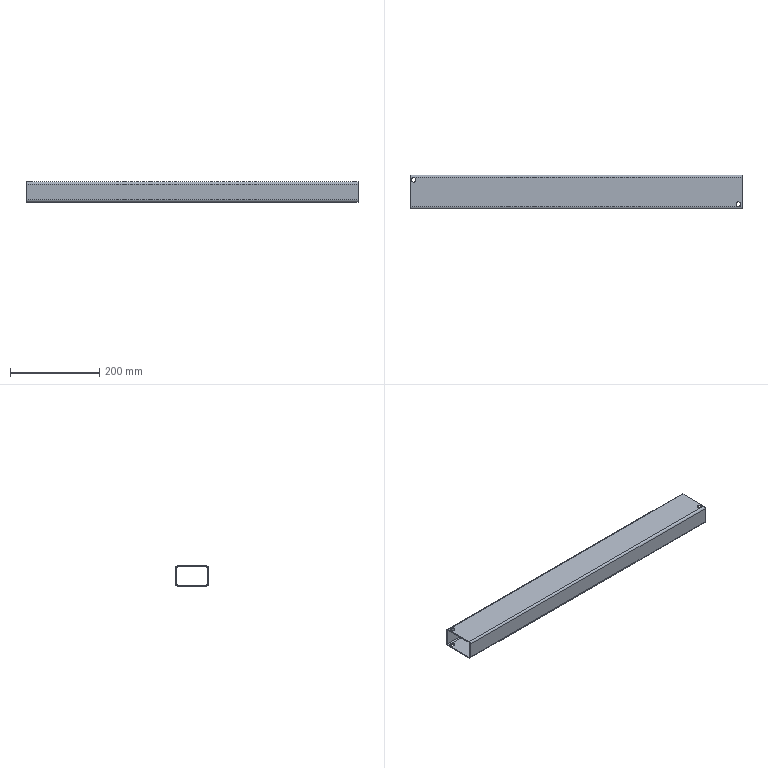Part | STEP file | [01]-4 | 1 solid | 28 faces | box 744 x 75 x 45 mm | volume 383906 mm3 | cylinder 18 | plane 10 | commonest cylinder face diameters 10 x10 4.6 x4 9.2 x4
STEP:
#1=CARTESIAN_POINT('',(613.,75.,17.5));
#2=VERTEX_POINT('',#1);
#3=CARTESIAN_POINT('',(613.,75.,27.5));
#4=VERTEX_POINT('',#3);
#5=CARTESIAN_POINT('',(613.,75.,22.5));
#6=DIRECTION('',(0.,-1.,0.));
#7=DIRECTION('',(0.,0.,1.));
#8=AXIS2_PLACEMENT_3D('',#5,#6,#7);
#9=CIRCLE('',#8,5.);
#10=EDGE_CURVE('',#2,#4,#9,.T.);
#11=ORIENTED_EDGE('',*,*,#10,.F.);
#12=CARTESIAN_POINT('',(613.,72.7,17.5));
#13=VERTEX_POINT('',#12);
#14=CARTESIAN_POINT('',(613.,75.,17.5));
#15=DIRECTION('',(0.,-1.,0.));
#16=VECTOR('',#15,1000.);
#17=LINE('',#14,#16);
#18=EDGE_CURVE('',#2,#13,#17,.T.);
#19=ORIENTED_EDGE('',*,*,#18,.T.);
#20=CARTESIAN_POINT('',(613.,72.7,27.5));
#21=VERTEX_POINT('',#20);
#22=CARTESIAN_POINT('',(613.,72.7,22.5));
#23=DIRECTION('',(0.,1.,0.));
#24=DIRECTION('',(0.,0.,-1.));
#25=AXIS2_PLACEMENT_3D('',#22,#23,#24);
#26=CIRCLE('',#25,5.);
#27=EDGE_CURVE('',#21,#13,#26,.T.);
#28=ORIENTED_EDGE('',*,*,#27,.F.);
#29=CARTESIAN_POINT('',(613.,75.,27.5));
#30=DIRECTION('',(0.,-1.,0.));
#31=VECTOR('',#30,1000.);
#32=LINE('',#29,#31);
#33=EDGE_CURVE('',#4,#21,#32,.T.);
#34=ORIENTED_EDGE('',*,*,#33,.F.);
#35=EDGE_LOOP('',(#11,#19,#28,#34));
#36=FACE_OUTER_BOUND('',#35,.T.);
#37=CARTESIAN_POINT('',(613.,75.,22.5));
#38=DIRECTION('',(0.,-1.,0.));
#39=DIRECTION('',(0.,0.,1.));
#40=AXIS2_PLACEMENT_3D('',#37,#38,#39);
#41=CYLINDRICAL_SURFACE('',#40,5.);
#42=ADVANCED_FACE('',(#36),#41,.F.);
#43=CARTESIAN_POINT('',(612.,5.5,42.7));
#44=VERTEX_POINT('',#43);
#45=CARTESIAN_POINT('',(612.,15.5,42.7));
#46=VERTEX_POINT('',#45);
#47=CARTESIAN_POINT('',(612.,10.5,42.7));
#48=DIRECTION('',(0.,0.,1.));
#49=DIRECTION('',(0.,1.,0.));
#50=AXIS2_PLACEMENT_3D('',#47,#48,#49);
#51=CIRCLE('',#50,5.);
#52=EDGE_CURVE('',#44,#46,#51,.T.);
#53=ORIENTED_EDGE('',*,*,#52,.F.);
#54=CARTESIAN_POINT('',(612.,5.5,45.));
#55=VERTEX_POINT('',#54);
#56=CARTESIAN_POINT('',(612.,5.5,42.7));
#57=DIRECTION('',(0.,0.,1.));
#58=VECTOR('',#57,1000.);
#59=LINE('',#56,#58);
#60=EDGE_CURVE('',#44,#55,#59,.T.);
#61=ORIENTED_EDGE('',*,*,#60,.T.);
#62=CARTESIAN_POINT('',(612.,15.5,45.));
#63=VERTEX_POINT('',#62);
#64=CARTESIAN_POINT('',(612.,10.5,45.));
#65=DIRECTION('',(0.,0.,-1.));
#66=DIRECTION('',(0.,-1.,0.));
#67=AXIS2_PLACEMENT_3D('',#64,#65,#66);
#68=CIRCLE('',#67,5.);
#69=EDGE_CURVE('',#63,#55,#68,.T.);
#70=ORIENTED_EDGE('',*,*,#69,.F.);
#71=CARTESIAN_POINT('',(612.,15.5,42.7));
#72=DIRECTION('',(0.,0.,1.));
#73=VECTOR('',#72,1000.);
#74=LINE('',#71,#73);
#75=EDGE_CURVE('',#46,#63,#74,.T.);
#76=ORIENTED_EDGE('',*,*,#75,.F.);
#77=EDGE_LOOP('',(#53,#61,#70,#76));
#78=FACE_OUTER_BOUND('',#77,.T.);
#79=CARTESIAN_POINT('',(612.,10.5,42.7));
#80=DIRECTION('',(0.,0.,1.));
#81=DIRECTION('',(0.,1.,0.));
#82=AXIS2_PLACEMENT_3D('',#79,#80,#81);
#83=CYLINDRICAL_SURFACE('',#82,5.);
#84=ADVANCED_FACE('',(#78),#83,.F.);
#85=CARTESIAN_POINT('',(-116.,69.5,2.3));
#86=VERTEX_POINT('',#85);
#87=CARTESIAN_POINT('',(-116.,59.5,2.3));
#88=VERTEX_POINT('',#87);
#89=CARTESIAN_POINT('',(-116.,64.5,2.3));
#90=DIRECTION('',(0.,0.,-1.));
#91=DIRECTION('',(0.,-1.,0.));
#92=AXIS2_PLACEMENT_3D('',#89,#90,#91);
#93=CIRCLE('',#92,5.);
#94=EDGE_CURVE('',#86,#88,#93,.T.);
#95=ORIENTED_EDGE('',*,*,#94,.F.);
#96=CARTESIAN_POINT('',(-116.,69.5,0.));
#97=VERTEX_POINT('',#96);
#98=CARTESIAN_POINT('',(-116.,69.5,2.3));
#99=DIRECTION('',(0.,0.,-1.));
#100=VECTOR('',#99,1000.);
#101=LINE('',#98,#100);
#102=EDGE_CURVE('',#86,#97,#101,.T.);
#103=ORIENTED_EDGE('',*,*,#102,.T.);
#104=CARTESIAN_POINT('',(-116.,59.5,0.));
#105=VERTEX_POINT('',#104);
#106=CARTESIAN_POINT('',(-116.,64.5,0.));
#107=DIRECTION('',(0.,0.,1.));
#108=DIRECTION('',(0.,1.,0.));
#109=AXIS2_PLACEMENT_3D('',#106,#107,#108);
#110=CIRCLE('',#109,5.);
#111=EDGE_CURVE('',#105,#97,#110,.T.);
#112=ORIENTED_EDGE('',*,*,#111,.F.);
#113=CARTESIAN_POINT('',(-116.,59.5,2.3));
#114=DIRECTION('',(0.,0.,-1.));
#115=VECTOR('',#114,1000.);
#116=LINE('',#113,#115);
#117=EDGE_CURVE('',#88,#105,#116,.T.);
#118=ORIENTED_EDGE('',*,*,#117,.F.);
#119=EDGE_LOOP('',(#95,#103,#112,#118));
#120=FACE_OUTER_BOUND('',#119,.T.);
#121=CARTESIAN_POINT('',(-116.,64.5,2.3));
#122=DIRECTION('',(0.,0.,-1.));
#123=DIRECTION('',(0.,-1.,0.));
#124=AXIS2_PLACEMENT_3D('',#121,#122,#123);
#125=CYLINDRICAL_SURFACE('',#124,5.);
#126=ADVANCED_FACE('',(#120),#125,.F.);
#127=CARTESIAN_POINT('',(612.,5.5,0.));
#128=VERTEX_POINT('',#127);
#129=CARTESIAN_POINT('',(612.,15.5,0.));
#130=VERTEX_POINT('',#129);
#131=CARTESIAN_POINT('',(612.,10.5,0.));
#132=DIRECTION('',(0.,0.,1.));
#133=DIRECTION('',(0.,1.,0.));
#134=AXIS2_PLACEMENT_3D('',#131,#132,#133);
#135=CIRCLE('',#134,5.);
#136=EDGE_CURVE('',#128,#130,#135,.T.);
#137=ORIENTED_EDGE('',*,*,#136,.F.);
#138=CARTESIAN_POINT('',(612.,5.5,2.3));
#139=VERTEX_POINT('',#138);
#140=CARTESIAN_POINT('',(612.,5.5,0.));
#141=DIRECTION('',(0.,0.,1.));
#142=VECTOR('',#141,1000.);
#143=LINE('',#140,#142);
#144=EDGE_CURVE('',#128,#139,#143,.T.);
#145=ORIENTED_EDGE('',*,*,#144,.T.);
#146=CARTESIAN_POINT('',(612.,15.5,2.3));
#147=VERTEX_POINT('',#146);
#148=CARTESIAN_POINT('',(612.,10.5,2.3));
#149=DIRECTION('',(0.,0.,-1.));
#150=DIRECTION('',(0.,-1.,0.));
#151=AXIS2_PLACEMENT_3D('',#148,#149,#150);
#152=CIRCLE('',#151,5.);
#153=EDGE_CURVE('',#147,#139,#152,.T.);
#154=ORIENTED_EDGE('',*,*,#153,.F.);
#155=CARTESIAN_POINT('',(612.,15.5,0.));
#156=DIRECTION('',(0.,0.,1.));
#157=VECTOR('',#156,1000.);
#158=LINE('',#155,#157);
#159=EDGE_CURVE('',#130,#147,#158,.T.);
#160=ORIENTED_EDGE('',*,*,#159,.F.);
#161=EDGE_LOOP('',(#137,#145,#154,#160));
#162=FACE_OUTER_BOUND('',#161,.T.);
#163=CARTESIAN_POINT('',(612.,10.5,0.));
#164=DIRECTION('',(0.,0.,1.));
#165=DIRECTION('',(0.,1.,0.));
#166=AXIS2_PLACEMENT_3D('',#163,#164,#165);
#167=CYLINDRICAL_SURFACE('',#166,5.);
#168=ADVANCED_FACE('',(#162),#167,.F.);
#169=CARTESIAN_POINT('',(-116.,69.5,45.));
#170=VERTEX_POINT('',#169);
#171=CARTESIAN_POINT('',(-116.,59.5,45.));
#172=VERTEX_POINT('',#171);
#173=CARTESIAN_POINT('',(-116.,64.5,45.));
#174=DIRECTION('',(0.,0.,-1.));
#175=DIRECTION('',(0.,-1.,0.));
#176=AXIS2_PLACEMENT_3D('',#173,#174,#175);
#177=CIRCLE('',#176,5.);
#178=EDGE_CURVE('',#170,#172,#177,.T.);
#179=ORIENTED_EDGE('',*,*,#178,.F.);
#180=CARTESIAN_POINT('',(-116.,69.5,42.7));
#181=VERTEX_POINT('',#180);
#182=CARTESIAN_POINT('',(-116.,69.5,45.));
#183=DIRECTION('',(0.,0.,-1.));
#184=VECTOR('',#183,1000.);
#185=LINE('',#182,#184);
#186=EDGE_CURVE('',#170,#181,#185,.T.);
#187=ORIENTED_EDGE('',*,*,#186,.T.);
#188=CARTESIAN_POINT('',(-116.,59.5,42.7));
#189=VERTEX_POINT('',#188);
#190=CARTESIAN_POINT('',(-116.,64.5,42.7));
#191=DIRECTION('',(0.,0.,1.));
#192=DIRECTION('',(0.,1.,0.));
#193=AXIS2_PLACEMENT_3D('',#190,#191,#192);
#194=CIRCLE('',#193,5.);
#195=EDGE_CURVE('',#189,#181,#194,.T.);
#196=ORIENTED_EDGE('',*,*,#195,.F.);
#197=CARTESIAN_POINT('',(-116.,59.5,45.));
#198=DIRECTION('',(0.,0.,-1.));
#199=VECTOR('',#198,1000.);
#200=LINE('',#197,#199);
#201=EDGE_CURVE('',#172,#189,#200,.T.);
#202=ORIENTED_EDGE('',*,*,#201,.F.);
#203=EDGE_LOOP('',(#179,#187,#196,#202));
#204=FACE_OUTER_BOUND('',#203,.T.);
#205=CARTESIAN_POINT('',(-116.,64.5,45.));
#206=DIRECTION('',(0.,0.,-1.));
#207=DIRECTION('',(0.,-1.,0.));
#208=AXIS2_PLACEMENT_3D('',#205,#206,#207);
#209=CYLINDRICAL_SURFACE('',#208,5.);
#210=ADVANCED_FACE('',(#204),#209,.F.);
#211=CARTESIAN_POINT('',(-124.,70.4,0.));
#212=VERTEX_POINT('',#211);
#213=CARTESIAN_POINT('',(-124.,4.6,0.));
#214=VERTEX_POINT('',#213);
#215=CARTESIAN_POINT('',(-124.,70.4,0.));
#216=DIRECTION('',(0.,-1.,0.));
#217=VECTOR('',#216,1000.);
#218=LINE('',#215,#217);
#219=EDGE_CURVE('',#212,#214,#218,.T.);
#220=ORIENTED_EDGE('',*,*,#219,.T.);
#221=CARTESIAN_POINT('',(-124.,0.,4.6));
#222=VERTEX_POINT('',#221);
#223=CARTESIAN_POINT('',(-124.,4.6,4.6));
#224=DIRECTION('',(-1.,0.,0.));
#225=DIRECTION('',(0.,0.,-1.));
#226=AXIS2_PLACEMENT_3D('',#223,#224,#225);
#227=CIRCLE('',#226,4.6);
#228=EDGE_CURVE('',#214,#222,#227,.T.);
#229=ORIENTED_EDGE('',*,*,#228,.T.);
#230=CARTESIAN_POINT('',(-124.,0.,40.4));
#231=VERTEX_POINT('',#230);
#232=CARTESIAN_POINT('',(-124.,0.,4.6));
#233=DIRECTION('',(0.,0.,1.));
#234=VECTOR('',#233,1000.);
#235=LINE('',#232,#234);
#236=EDGE_CURVE('',#222,#231,#235,.T.);
#237=ORIENTED_EDGE('',*,*,#236,.T.);
#238=CARTESIAN_POINT('',(-124.,4.6,45.));
#239=VERTEX_POINT('',#238);
#240=CARTESIAN_POINT('',(-124.,4.6,40.4));
#241=DIRECTION('',(-1.,0.,0.));
#242=DIRECTION('',(0.,0.,-1.));
#243=AXIS2_PLACEMENT_3D('',#240,#241,#242);
#244=CIRCLE('',#243,4.6);
#245=EDGE_CURVE('',#231,#239,#244,.T.);
#246=ORIENTED_EDGE('',*,*,#245,.T.);
#247=CARTESIAN_POINT('',(-124.,70.4,45.));
#248=VERTEX_POINT('',#247);
#249=CARTESIAN_POINT('',(-124.,4.6,45.));
#250=DIRECTION('',(0.,1.,0.));
#251=VECTOR('',#250,1000.);
#252=LINE('',#249,#251);
#253=EDGE_CURVE('',#239,#248,#252,.T.);
#254=ORIENTED_EDGE('',*,*,#253,.T.);
#255=CARTESIAN_POINT('',(-124.,75.,40.4));
#256=VERTEX_POINT('',#255);
#257=CARTESIAN_POINT('',(-124.,70.4,40.4));
#258=DIRECTION('',(-1.,0.,0.));
#259=DIRECTION('',(0.,0.,-1.));
#260=AXIS2_PLACEMENT_3D('',#257,#258,#259);
#261=CIRCLE('',#260,4.6);
#262=EDGE_CURVE('',#248,#256,#261,.T.);
#263=ORIENTED_EDGE('',*,*,#262,.T.);
#264=CARTESIAN_POINT('',(-124.,75.,4.6));
#265=VERTEX_POINT('',#264);
#266=CARTESIAN_POINT('',(-124.,75.,40.4));
#267=DIRECTION('',(0.,0.,-1.));
#268=VECTOR('',#267,1000.);
#269=LINE('',#266,#268);
#270=EDGE_CURVE('',#256,#265,#269,.T.);
#271=ORIENTED_EDGE('',*,*,#270,.T.);
#272=CARTESIAN_POINT('',(-124.,70.4,4.6));
#273=DIRECTION('',(-1.,0.,0.));
#274=DIRECTION('',(0.,0.,-1.));
#275=AXIS2_PLACEMENT_3D('',#272,#273,#274);
#276=CIRCLE('',#275,4.6);
#277=EDGE_CURVE('',#265,#212,#276,.T.);
#278=ORIENTED_EDGE('',*,*,#277,.T.);
#279=EDGE_LOOP('',(#220,#229,#237,#246,#254,#263,#271,#278));
#280=FACE_OUTER_BOUND('',#279,.T.);
#281=CARTESIAN_POINT('',(-124.,70.4,2.3));
#282=VERTEX_POINT('',#281);
#283=CARTESIAN_POINT('',(-124.,4.6,2.3));
#284=VERTEX_POINT('',#283);
#285=CARTESIAN_POINT('',(-124.,70.4,2.3));
#286=DIRECTION('',(0.,-1.,0.));
#287=VECTOR('',#286,1000.);
#288=LINE('',#285,#287);
#289=EDGE_CURVE('',#282,#284,#288,.T.);
#290=ORIENTED_EDGE('',*,*,#289,.F.);
#291=CARTESIAN_POINT('',(-124.,72.7,4.6));
#292=VERTEX_POINT('',#291);
#293=CARTESIAN_POINT('',(-124.,70.4,4.6));
#294=DIRECTION('',(-1.,0.,0.));
#295=DIRECTION('',(0.,1.,0.));
#296=AXIS2_PLACEMENT_3D('',#293,#294,#295);
#297=CIRCLE('',#296,2.3);
#298=EDGE_CURVE('',#292,#282,#297,.T.);
#299=ORIENTED_EDGE('',*,*,#298,.F.);
#300=CARTESIAN_POINT('',(-124.,72.7,40.4));
#301=VERTEX_POINT('',#300);
#302=CARTESIAN_POINT('',(-124.,72.7,40.4));
#303=DIRECTION('',(0.,0.,-1.));
#304=VECTOR('',#303,1000.);
#305=LINE('',#302,#304);
#306=EDGE_CURVE('',#301,#292,#305,.T.);
#307=ORIENTED_EDGE('',*,*,#306,.F.);
#308=CARTESIAN_POINT('',(-124.,70.4,42.7));
#309=VERTEX_POINT('',#308);
#310=CARTESIAN_POINT('',(-124.,70.4,40.4));
#311=DIRECTION('',(-1.,0.,0.));
#312=DIRECTION('',(0.,1.,0.));
#313=AXIS2_PLACEMENT_3D('',#310,#311,#312);
#314=CIRCLE('',#313,2.3);
#315=EDGE_CURVE('',#309,#301,#314,.T.);
#316=ORIENTED_EDGE('',*,*,#315,.F.);
#317=CARTESIAN_POINT('',(-124.,4.6,42.7));
#318=VERTEX_POINT('',#317);
#319=CARTESIAN_POINT('',(-124.,4.6,42.7));
#320=DIRECTION('',(0.,1.,0.));
#321=VECTOR('',#320,1000.);
#322=LINE('',#319,#321);
#323=EDGE_CURVE('',#318,#309,#322,.T.);
#324=ORIENTED_EDGE('',*,*,#323,.F.);
#325=CARTESIAN_POINT('',(-124.,2.3,40.4));
#326=VERTEX_POINT('',#325);
#327=CARTESIAN_POINT('',(-124.,4.6,40.4));
#328=DIRECTION('',(-1.,0.,0.));
#329=DIRECTION('',(0.,1.,0.));
#330=AXIS2_PLACEMENT_3D('',#327,#328,#329);
#331=CIRCLE('',#330,2.3);
#332=EDGE_CURVE('',#326,#318,#331,.T.);
#333=ORIENTED_EDGE('',*,*,#332,.F.);
#334=CARTESIAN_POINT('',(-124.,2.3,4.6));
#335=VERTEX_POINT('',#334);
#336=CARTESIAN_POINT('',(-124.,2.3,4.6));
#337=DIRECTION('',(0.,0.,1.));
#338=VECTOR('',#337,1000.);
#339=LINE('',#336,#338);
#340=EDGE_CURVE('',#335,#326,#339,.T.);
#341=ORIENTED_EDGE('',*,*,#340,.F.);
#342=CARTESIAN_POINT('',(-124.,4.6,4.6));
#343=DIRECTION('',(-1.,0.,0.));
#344=DIRECTION('',(0.,1.,0.));
#345=AXIS2_PLACEMENT_3D('',#342,#343,#344);
#346=CIRCLE('',#345,2.3);
#347=EDGE_CURVE('',#284,#335,#346,.T.);
#348=ORIENTED_EDGE('',*,*,#347,.F.);
#349=EDGE_LOOP('',(#290,#299,#307,#316,#324,#333,#341,#348));
#350=FACE_BOUND('',#349,.T.);
#351=CARTESIAN_POINT('',(-124.,4.6,4.6));
#352=DIRECTION('',(-1.,0.,0.));
#353=DIRECTION('',(0.,0.,-1.));
#354=AXIS2_PLACEMENT_3D('',#351,#352,#353);
#355=PLANE('',#354);
#356=ADVANCED_FACE('',(#280,#350),#355,.T.);
#357=CARTESIAN_POINT('',(620.,70.4,0.));
#358=VERTEX_POINT('',#357);
#359=CARTESIAN_POINT('',(620.,4.6,0.));
#360=VERTEX_POINT('',#359);
#361=CARTESIAN_POINT('',(620.,70.4,0.));
#362=DIRECTION('',(0.,-1.,0.));
#363=VECTOR('',#362,1000.);
#364=LINE('',#361,#363);
#365=EDGE_CURVE('',#358,#360,#364,.T.);
#366=ORIENTED_EDGE('',*,*,#365,.F.);
#367=CARTESIAN_POINT('',(620.,75.,4.6));
#368=VERTEX_POINT('',#367);
#369=CARTESIAN_POINT('',(620.,70.4,4.6));
#370=DIRECTION('',(-1.,0.,0.));
#371=DIRECTION('',(0.,0.,-1.));
#372=AXIS2_PLACEMENT_3D('',#369,#370,#371);
#373=CIRCLE('',#372,4.6);
#374=EDGE_CURVE('',#368,#358,#373,.T.);
#375=ORIENTED_EDGE('',*,*,#374,.F.);
#376=CARTESIAN_POINT('',(620.,75.,40.4));
#377=VERTEX_POINT('',#376);
#378=CARTESIAN_POINT('',(620.,75.,40.4));
#379=DIRECTION('',(0.,0.,-1.));
#380=VECTOR('',#379,1000.);
#381=LINE('',#378,#380);
#382=EDGE_CURVE('',#377,#368,#381,.T.);
#383=ORIENTED_EDGE('',*,*,#382,.F.);
#384=CARTESIAN_POINT('',(620.,70.4,45.));
#385=VERTEX_POINT('',#384);
#386=CARTESIAN_POINT('',(620.,70.4,40.4));
#387=DIRECTION('',(-1.,0.,0.));
#388=DIRECTION('',(0.,0.,-1.));
#389=AXIS2_PLACEMENT_3D('',#386,#387,#388);
#390=CIRCLE('',#389,4.6);
#391=EDGE_CURVE('',#385,#377,#390,.T.);
#392=ORIENTED_EDGE('',*,*,#391,.F.);
#393=CARTESIAN_POINT('',(620.,4.6,45.));
#394=VERTEX_POINT('',#393);
#395=CARTESIAN_POINT('',(620.,4.6,45.));
#396=DIRECTION('',(0.,1.,0.));
#397=VECTOR('',#396,1000.);
#398=LINE('',#395,#397);
#399=EDGE_CURVE('',#394,#385,#398,.T.);
#400=ORIENTED_EDGE('',*,*,#399,.F.);
#401=CARTESIAN_POINT('',(620.,0.,40.4));
#402=VERTEX_POINT('',#401);
#403=CARTESIAN_POINT('',(620.,4.6,40.4));
#404=DIRECTION('',(-1.,0.,0.));
#405=DIRECTION('',(0.,0.,-1.));
#406=AXIS2_PLACEMENT_3D('',#403,#404,#405);
#407=CIRCLE('',#406,4.6);
#408=EDGE_CURVE('',#402,#394,#407,.T.);
#409=ORIENTED_EDGE('',*,*,#408,.F.);
#410=CARTESIAN_POINT('',(620.,0.,4.6));
#411=VERTEX_POINT('',#410);
#412=CARTESIAN_POINT('',(620.,0.,4.6));
#413=DIRECTION('',(0.,0.,1.));
#414=VECTOR('',#413,1000.);
#415=LINE('',#412,#414);
#416=EDGE_CURVE('',#411,#402,#415,.T.);
#417=ORIENTED_EDGE('',*,*,#416,.F.);
#418=CARTESIAN_POINT('',(620.,4.6,4.6));
#419=DIRECTION('',(-1.,0.,0.));
#420=DIRECTION('',(0.,0.,-1.));
#421=AXIS2_PLACEMENT_3D('',#418,#419,#420);
#422=CIRCLE('',#421,4.6);
#423=EDGE_CURVE('',#360,#411,#422,.T.);
#424=ORIENTED_EDGE('',*,*,#423,.F.);
#425=EDGE_LOOP('',(#366,#375,#383,#392,#400,#409,#417,#424));
#426=FACE_OUTER_BOUND('',#425,.T.);
#427=CARTESIAN_POINT('',(620.,72.7,4.6));
#428=VERTEX_POINT('',#427);
#429=CARTESIAN_POINT('',(620.,70.4,2.3));
#430=VERTEX_POINT('',#429);
#431=CARTESIAN_POINT('',(620.,70.4,4.6));
#432=DIRECTION('',(-1.,0.,0.));
#433=DIRECTION('',(0.,1.,0.));
#434=AXIS2_PLACEMENT_3D('',#431,#432,#433);
#435=CIRCLE('',#434,2.3);
#436=EDGE_CURVE('',#428,#430,#435,.T.);
#437=ORIENTED_EDGE('',*,*,#436,.T.);
#438=CARTESIAN_POINT('',(620.,4.6,2.3));
#439=VERTEX_POINT('',#438);
#440=CARTESIAN_POINT('',(620.,70.4,2.3));
#441=DIRECTION('',(0.,-1.,0.));
#442=VECTOR('',#441,1000.);
#443=LINE('',#440,#442);
#444=EDGE_CURVE('',#430,#439,#443,.T.);
#445=ORIENTED_EDGE('',*,*,#444,.T.);
#446=CARTESIAN_POINT('',(620.,2.3,4.6));
#447=VERTEX_POINT('',#446);
#448=CARTESIAN_POINT('',(620.,4.6,4.6));
#449=DIRECTION('',(-1.,0.,0.));
#450=DIRECTION('',(0.,1.,0.));
#451=AXIS2_PLACEMENT_3D('',#448,#449,#450);
#452=CIRCLE('',#451,2.3);
#453=EDGE_CURVE('',#439,#447,#452,.T.);
#454=ORIENTED_EDGE('',*,*,#453,.T.);
#455=CARTESIAN_POINT('',(620.,2.3,40.4));
#456=VERTEX_POINT('',#455);
#457=CARTESIAN_POINT('',(620.,2.3,4.6));
#458=DIRECTION('',(0.,0.,1.));
#459=VECTOR('',#458,1000.);
#460=LINE('',#457,#459);
#461=EDGE_CURVE('',#447,#456,#460,.T.);
#462=ORIENTED_EDGE('',*,*,#461,.T.);
#463=CARTESIAN_POINT('',(620.,4.6,42.7));
#464=VERTEX_POINT('',#463);
#465=CARTESIAN_POINT('',(620.,4.6,40.4));
#466=DIRECTION('',(-1.,0.,0.));
#467=DIRECTION('',(0.,1.,0.));
#468=AXIS2_PLACEMENT_3D('',#465,#466,#467);
#469=CIRCLE('',#468,2.3);
#470=EDGE_CURVE('',#456,#464,#469,.T.);
#471=ORIENTED_EDGE('',*,*,#470,.T.);
#472=CARTESIAN_POINT('',(620.,70.4,42.7));
#473=VERTEX_POINT('',#472);
#474=CARTESIAN_POINT('',(620.,4.6,42.7));
#475=DIRECTION('',(0.,1.,0.));
#476=VECTOR('',#475,1000.);
#477=LINE('',#474,#476);
#478=EDGE_CURVE('',#464,#473,#477,.T.);
#479=ORIENTED_EDGE('',*,*,#478,.T.);
#480=CARTESIAN_POINT('',(620.,72.7,40.4));
#481=VERTEX_POINT('',#480);
#482=CARTESIAN_POINT('',(620.,70.4,40.4));
#483=DIRECTION('',(-1.,0.,0.));
#484=DIRECTION('',(0.,1.,0.));
#485=AXIS2_PLACEMENT_3D('',#482,#483,#484);
#486=CIRCLE('',#485,2.3);
#487=EDGE_CURVE('',#473,#481,#486,.T.);
#488=ORIENTED_EDGE('',*,*,#487,.T.);
#489=CARTESIAN_POINT('',(620.,72.7,40.4));
#490=DIRECTION('',(0.,0.,-1.));
#491=VECTOR('',#490,1000.);
#492=LINE('',#489,#491);
#493=EDGE_CURVE('',#481,#428,#492,.T.);
#494=ORIENTED_EDGE('',*,*,#493,.T.);
#495=EDGE_LOOP('',(#437,#445,#454,#462,#471,#479,#488,#494));
#496=FACE_BOUND('',#495,.T.);
#497=CARTESIAN_POINT('',(620.,4.6,4.6));
#498=DIRECTION('',(-1.,0.,0.));
#499=DIRECTION('',(0.,0.,-1.));
#500=AXIS2_PLACEMENT_3D('',#497,#498,#499);
#501=PLANE('',#500);
#502=ADVANCED_FACE('',(#426,#496),#501,.F.);
#503=ORIENTED_EDGE('',*,*,#111,.T.);
#504=CARTESIAN_POINT('',(-116.,64.5,0.));
#505=DIRECTION('',(0.,0.,1.));
#506=DIRECTION('',(0.,1.,0.));
#507=AXIS2_PLACEMENT_3D('',#504,#505,#506);
#508=CIRCLE('',#507,5.);
#509=EDGE_CURVE('',#97,#105,#508,.T.);
#510=ORIENTED_EDGE('',*,*,#509,.T.);
#511=EDGE_LOOP('',(#503,#510));
#512=FACE_BOUND('',#511,.T.);
#513=CARTESIAN_POINT('',(612.,10.5,0.));
#514=DIRECTION('',(0.,0.,1.));
#515=DIRECTION('',(0.,1.,0.));
#516=AXIS2_PLACEMENT_3D('',#513,#514,#515);
#517=CIRCLE('',#516,5.);
#518=EDGE_CURVE('',#130,#128,#517,.T.);
#519=ORIENTED_EDGE('',*,*,#518,.T.);
#520=ORIENTED_EDGE('',*,*,#136,.T.);
#521=EDGE_LOOP('',(#519,#520));
#522=FACE_BOUND('',#521,.T.);
#523=ORIENTED_EDGE('',*,*,#365,.T.);
#524=CARTESIAN_POINT('',(-124.,4.6,0.));
#525=DIRECTION('',(1.,0.,0.));
#526=VECTOR('',#525,1000.);
#527=LINE('',#524,#526);
#528=EDGE_CURVE('',#214,#360,#527,.T.);
#529=ORIENTED_EDGE('',*,*,#528,.F.);
#530=ORIENTED_EDGE('',*,*,#219,.F.);
#531=CARTESIAN_POINT('',(-124.,70.4,0.));
#532=DIRECTION('',(1.,0.,0.));
#533=VECTOR('',#532,1000.);
#534=LINE('',#531,#533);
#535=EDGE_CURVE('',#212,#358,#534,.T.);
#536=ORIENTED_EDGE('',*,*,#535,.T.);
#537=EDGE_LOOP('',(#523,#529,#530,#536));
#538=FACE_OUTER_BOUND('',#537,.T.);
#539=CARTESIAN_POINT('',(-124.,70.4,0.));
#540=DIRECTION('',(0.,0.,1.));
#541=DIRECTION('',(0.,1.,0.));
#542=AXIS2_PLACEMENT_3D('',#539,#540,#541);
#543=PLANE('',#542);
#544=ADVANCED_FACE('',(#512,#522,#538),#543,.F.);
#545=ORIENTED_EDGE('',*,*,#423,.T.);
#546=CARTESIAN_POINT('',(-124.,0.,4.6));
#547=DIRECTION('',(1.,0.,0.));
#548=VECTOR('',#547,1000.);
#549=LINE('',#546,#548);
#550=EDGE_CURVE('',#222,#411,#549,.T.);
#551=ORIENTED_EDGE('',*,*,#550,.F.);
#552=ORIENTED_EDGE('',*,*,#228,.F.);
#553=ORIENTED_EDGE('',*,*,#528,.T.);
#554=EDGE_LOOP('',(#545,#551,#552,#553));
#555=FACE_OUTER_BOUND('',#554,.T.);
#556=CARTESIAN_POINT('',(-124.,4.6,4.6));
#557=DIRECTION('',(1.,0.,0.));
#558=DIRECTION('',(0.,0.,1.));
#559=AXIS2_PLACEMENT_3D('',#556,#557,#558);
#560=CYLINDRICAL_SURFACE('',#559,4.6);
#561=ADVANCED_FACE('',(#555),#560,.T.);
#562=ORIENTED_EDGE('',*,*,#416,.T.);
#563=CARTESIAN_POINT('',(-124.,0.,40.4));
#564=DIRECTION('',(1.,0.,0.));
#565=VECTOR('',#564,1000.);
#566=LINE('',#563,#565);
#567=EDGE_CURVE('',#231,#402,#566,.T.);
#568=ORIENTED_EDGE('',*,*,#567,.F.);
#569=ORIENTED_EDGE('',*,*,#236,.F.);
#570=ORIENTED_EDGE('',*,*,#550,.T.);
#571=EDGE_LOOP('',(#562,#568,#569,#570));
#572=FACE_OUTER_BOUND('',#571,.T.);
#573=CARTESIAN_POINT('',(-124.,0.,4.6));
#574=DIRECTION('',(0.,1.,0.));
#575=DIRECTION('',(0.,0.,-1.));
#576=AXIS2_PLACEMENT_3D('',#573,#574,#575);
#577=PLANE('',#576);
#578=ADVANCED_FACE('',(#572),#577,.F.);
#579=ORIENTED_EDGE('',*,*,#408,.T.);
#580=CARTESIAN_POINT('',(-124.,4.6,45.));
#581=DIRECTION('',(1.,0.,0.));
#582=VECTOR('',#581,1000.);
#583=LINE('',#580,#582);
#584=EDGE_CURVE('',#239,#394,#583,.T.);
#585=ORIENTED_EDGE('',*,*,#584,.F.);
#586=ORIENTED_EDGE('',*,*,#245,.F.);
#587=ORIENTED_EDGE('',*,*,#567,.T.);
#588=EDGE_LOOP('',(#579,#585,#586,#587));
#589=FACE_OUTER_BOUND('',#588,.T.);
#590=CARTESIAN_POINT('',(-124.,4.6,40.4));
#591=DIRECTION('',(1.,0.,0.));
#592=DIRECTION('',(0.,0.,1.));
#593=AXIS2_PLACEMENT_3D('',#590,#591,#592);
#594=CYLINDRICAL_SURFACE('',#593,4.6);
#595=ADVANCED_FACE('',(#589),#594,.T.);
#596=ORIENTED_EDGE('',*,*,#69,.T.);
#597=CARTESIAN_POINT('',(612.,10.5,45.));
#598=DIRECTION('',(0.,0.,-1.));
#599=DIRECTION('',(0.,-1.,0.));
#600=AXIS2_PLACEMENT_3D('',#597,#598,#599);
#601=CIRCLE('',#600,5.);
#602=EDGE_CURVE('',#55,#63,#601,.T.);
#603=ORIENTED_EDGE('',*,*,#602,.T.);
#604=EDGE_LOOP('',(#596,#603));
#605=FACE_BOUND('',#604,.T.);
#606=CARTESIAN_POINT('',(-116.,64.5,45.));
#607=DIRECTION('',(0.,0.,-1.));
#608=DIRECTION('',(0.,-1.,0.));
#609=AXIS2_PLACEMENT_3D('',#606,#607,#608);
#610=CIRCLE('',#609,5.);
#611=EDGE_CURVE('',#172,#170,#610,.T.);
#612=ORIENTED_EDGE('',*,*,#611,.T.);
#613=ORIENTED_EDGE('',*,*,#178,.T.);
#614=EDGE_LOOP('',(#612,#613));
#615=FACE_BOUND('',#614,.T.);
#616=ORIENTED_EDGE('',*,*,#399,.T.);
#617=CARTESIAN_POINT('',(-124.,70.4,45.));
#618=DIRECTION('',(1.,0.,0.));
#619=VECTOR('',#618,1000.);
#620=LINE('',#617,#619);
#621=EDGE_CURVE('',#248,#385,#620,.T.);
#622=ORIENTED_EDGE('',*,*,#621,.F.);
#623=ORIENTED_EDGE('',*,*,#253,.F.);
#624=ORIENTED_EDGE('',*,*,#584,.T.);
#625=EDGE_LOOP('',(#616,#622,#623,#624));
#626=FACE_OUTER_BOUND('',#625,.T.);
#627=CARTESIAN_POINT('',(-124.,4.6,45.));
#628=DIRECTION('',(0.,0.,-1.));
#629=DIRECTION('',(0.,-1.,0.));
#630=AXIS2_PLACEMENT_3D('',#627,#628,#629);
#631=PLANE('',#630);
#632=ADVANCED_FACE('',(#605,#615,#626),#631,.F.);
#633=ORIENTED_EDGE('',*,*,#391,.T.);
#634=CARTESIAN_POINT('',(-124.,75.,40.4));
#635=DIRECTION('',(1.,0.,0.));
#636=VECTOR('',#635,1000.);
#637=LINE('',#634,#636);
#638=EDGE_CURVE('',#256,#377,#637,.T.);
#639=ORIENTED_EDGE('',*,*,#638,.F.);
#640=ORIENTED_EDGE('',*,*,#262,.F.);
#641=ORIENTED_EDGE('',*,*,#621,.T.);
#642=EDGE_LOOP('',(#633,#639,#640,#641));
#643=FACE_OUTER_BOUND('',#642,.T.);
#644=CARTESIAN_POINT('',(-124.,70.4,40.4));
#645=DIRECTION('',(1.,0.,0.));
#646=DIRECTION('',(0.,0.,1.));
#647=AXIS2_PLACEMENT_3D('',#644,#645,#646);
#648=CYLINDRICAL_SURFACE('',#647,4.6);
#649=ADVANCED_FACE('',(#643),#648,.T.);
#650=CARTESIAN_POINT('',(613.,75.,22.5));
#651=DIRECTION('',(0.,-1.,0.));
#652=DIRECTION('',(0.,0.,1.));
#653=AXIS2_PLACEMENT_3D('',#650,#651,#652);
#654=CIRCLE('',#653,5.);
#655=EDGE_CURVE('',#4,#2,#654,.T.);
#656=ORIENTED_EDGE('',*,*,#655,.T.);
#657=ORIENTED_EDGE('',*,*,#10,.T.);
#658=EDGE_LOOP('',(#656,#657));
#659=FACE_BOUND('',#658,.T.);
#660=ORIENTED_EDGE('',*,*,#382,.T.);
#661=CARTESIAN_POINT('',(-124.,75.,4.6));
#662=DIRECTION('',(1.,0.,0.));
#663=VECTOR('',#662,1000.);
#664=LINE('',#661,#663);
#665=EDGE_CURVE('',#265,#368,#664,.T.);
#666=ORIENTED_EDGE('',*,*,#665,.F.);
#667=ORIENTED_EDGE('',*,*,#270,.F.);
#668=ORIENTED_EDGE('',*,*,#638,.T.);
#669=EDGE_LOOP('',(#660,#666,#667,#668));
#670=FACE_OUTER_BOUND('',#669,.T.);
#671=CARTESIAN_POINT('',(-124.,75.,40.4));
#672=DIRECTION('',(0.,-1.,0.));
#673=DIRECTION('',(-1.,0.,0.));
#674=AXIS2_PLACEMENT_3D('',#671,#672,#673);
#675=PLANE('',#674);
#676=ADVANCED_FACE('',(#659,#670),#675,.F.);
#677=ORIENTED_EDGE('',*,*,#374,.T.);
#678=ORIENTED_EDGE('',*,*,#535,.F.);
#679=ORIENTED_EDGE('',*,*,#277,.F.);
#680=ORIENTED_EDGE('',*,*,#665,.T.);
#681=EDGE_LOOP('',(#677,#678,#679,#680));
#682=FACE_OUTER_BOUND('',#681,.T.);
#683=CARTESIAN_POINT('',(-124.,70.4,4.6));
#684=DIRECTION('',(1.,0.,0.));
#685=DIRECTION('',(0.,0.,1.));
#686=AXIS2_PLACEMENT_3D('',#683,#684,#685);
#687=CYLINDRICAL_SURFACE('',#686,4.6);
#688=ADVANCED_FACE('',(#682),#687,.T.);
#689=ORIENTED_EDGE('',*,*,#436,.F.);
#690=CARTESIAN_POINT('',(-124.,72.7,4.6));
#691=DIRECTION('',(1.,0.,0.));
#692=VECTOR('',#691,1000.);
#693=LINE('',#690,#692);
#694=EDGE_CURVE('',#292,#428,#693,.T.);
#695=ORIENTED_EDGE('',*,*,#694,.F.);
#696=ORIENTED_EDGE('',*,*,#298,.T.);
#697=CARTESIAN_POINT('',(-124.,70.4,2.3));
#698=DIRECTION('',(1.,0.,0.));
#699=VECTOR('',#698,1000.);
#700=LINE('',#697,#699);
#701=EDGE_CURVE('',#282,#430,#700,.T.);
#702=ORIENTED_EDGE('',*,*,#701,.T.);
#703=EDGE_LOOP('',(#689,#695,#696,#702));
#704=FACE_OUTER_BOUND('',#703,.T.);
#705=CARTESIAN_POINT('',(-124.,70.4,4.6));
#706=DIRECTION('',(1.,0.,0.));
#707=DIRECTION('',(0.,-1.,0.));
#708=AXIS2_PLACEMENT_3D('',#705,#706,#707);
#709=CYLINDRICAL_SURFACE('',#708,2.3);
#710=ADVANCED_FACE('',(#704),#709,.F.);
#711=CARTESIAN_POINT('',(-116.,64.5,2.3));
#712=DIRECTION('',(0.,0.,-1.));
#713=DIRECTION('',(0.,-1.,0.));
#714=AXIS2_PLACEMENT_3D('',#711,#712,#713);
#715=CIRCLE('',#714,5.);
#716=EDGE_CURVE('',#88,#86,#715,.T.);
#717=ORIENTED_EDGE('',*,*,#716,.T.);
#718=ORIENTED_EDGE('',*,*,#94,.T.);
#719=EDGE_LOOP('',(#717,#718));
#720=FACE_BOUND('',#719,.T.);
#721=ORIENTED_EDGE('',*,*,#153,.T.);
#722=CARTESIAN_POINT('',(612.,10.5,2.3));
#723=DIRECTION('',(0.,0.,-1.));
#724=DIRECTION('',(0.,-1.,0.));
#725=AXIS2_PLACEMENT_3D('',#722,#723,#724);
#726=CIRCLE('',#725,5.);
#727=EDGE_CURVE('',#139,#147,#726,.T.);
#728=ORIENTED_EDGE('',*,*,#727,.T.);
#729=EDGE_LOOP('',(#721,#728));
#730=FACE_BOUND('',#729,.T.);
#731=ORIENTED_EDGE('',*,*,#444,.F.);
#732=ORIENTED_EDGE('',*,*,#701,.F.);
#733=ORIENTED_EDGE('',*,*,#289,.T.);
#734=CARTESIAN_POINT('',(-124.,4.6,2.3));
#735=DIRECTION('',(1.,0.,0.));
#736=VECTOR('',#735,1000.);
#737=LINE('',#734,#736);
#738=EDGE_CURVE('',#284,#439,#737,.T.);
#739=ORIENTED_EDGE('',*,*,#738,.T.);
#740=EDGE_LOOP('',(#731,#732,#733,#739));
#741=FACE_OUTER_BOUND('',#740,.T.);
#742=CARTESIAN_POINT('',(-124.,70.4,2.3));
#743=DIRECTION('',(0.,0.,1.));
#744=DIRECTION('',(1.,0.,0.));
#745=AXIS2_PLACEMENT_3D('',#742,#743,#744);
#746=PLANE('',#745);
#747=ADVANCED_FACE('',(#720,#730,#741),#746,.T.);
#748=ORIENTED_EDGE('',*,*,#453,.F.);
#749=ORIENTED_EDGE('',*,*,#738,.F.);
#750=ORIENTED_EDGE('',*,*,#347,.T.);
#751=CARTESIAN_POINT('',(-124.,2.3,4.6));
#752=DIRECTION('',(1.,0.,0.));
#753=VECTOR('',#752,1000.);
#754=LINE('',#751,#753);
#755=EDGE_CURVE('',#335,#447,#754,.T.);
#756=ORIENTED_EDGE('',*,*,#755,.T.);
#757=EDGE_LOOP('',(#748,#749,#750,#756));
#758=FACE_OUTER_BOUND('',#757,.T.);
#759=CARTESIAN_POINT('',(-124.,4.6,4.6));
#760=DIRECTION('',(1.,0.,0.));
#761=DIRECTION('',(0.,-1.,0.));
#762=AXIS2_PLACEMENT_3D('',#759,#760,#761);
#763=CYLINDRICAL_SURFACE('',#762,2.3);
#764=ADVANCED_FACE('',(#758),#763,.F.);
#765=ORIENTED_EDGE('',*,*,#461,.F.);
#766=ORIENTED_EDGE('',*,*,#755,.F.);
#767=ORIENTED_EDGE('',*,*,#340,.T.);
#768=CARTESIAN_POINT('',(-124.,2.3,40.4));
#769=DIRECTION('',(1.,0.,0.));
#770=VECTOR('',#769,1000.);
#771=LINE('',#768,#770);
#772=EDGE_CURVE('',#326,#456,#771,.T.);
#773=ORIENTED_EDGE('',*,*,#772,.T.);
#774=EDGE_LOOP('',(#765,#766,#767,#773));
#775=FACE_OUTER_BOUND('',#774,.T.);
#776=CARTESIAN_POINT('',(-124.,2.3,4.6));
#777=DIRECTION('',(0.,1.,0.));
#778=DIRECTION('',(1.,0.,0.));
#779=AXIS2_PLACEMENT_3D('',#776,#777,#778);
#780=PLANE('',#779);
#781=ADVANCED_FACE('',(#775),#780,.T.);
#782=ORIENTED_EDGE('',*,*,#470,.F.);
#783=ORIENTED_EDGE('',*,*,#772,.F.);
#784=ORIENTED_EDGE('',*,*,#332,.T.);
#785=CARTESIAN_POINT('',(-124.,4.6,42.7));
#786=DIRECTION('',(1.,0.,0.));
#787=VECTOR('',#786,1000.);
#788=LINE('',#785,#787);
#789=EDGE_CURVE('',#318,#464,#788,.T.);
#790=ORIENTED_EDGE('',*,*,#789,.T.);
#791=EDGE_LOOP('',(#782,#783,#784,#790));
#792=FACE_OUTER_BOUND('',#791,.T.);
#793=CARTESIAN_POINT('',(-124.,4.6,40.4));
#794=DIRECTION('',(1.,0.,0.));
#795=DIRECTION('',(0.,-1.,0.));
#796=AXIS2_PLACEMENT_3D('',#793,#794,#795);
#797=CYLINDRICAL_SURFACE('',#796,2.3);
#798=ADVANCED_FACE('',(#792),#797,.F.);
#799=CARTESIAN_POINT('',(612.,10.5,42.7));
#800=DIRECTION('',(0.,0.,1.));
#801=DIRECTION('',(0.,1.,0.));
#802=AXIS2_PLACEMENT_3D('',#799,#800,#801);
#803=CIRCLE('',#802,5.);
#804=EDGE_CURVE('',#46,#44,#803,.T.);
#805=ORIENTED_EDGE('',*,*,#804,.T.);
#806=ORIENTED_EDGE('',*,*,#52,.T.);
#807=EDGE_LOOP('',(#805,#806));
#808=FACE_BOUND('',#807,.T.);
#809=ORIENTED_EDGE('',*,*,#195,.T.);
#810=CARTESIAN_POINT('',(-116.,64.5,42.7));
#811=DIRECTION('',(0.,0.,1.));
#812=DIRECTION('',(0.,1.,0.));
#813=AXIS2_PLACEMENT_3D('',#810,#811,#812);
#814=CIRCLE('',#813,5.);
#815=EDGE_CURVE('',#181,#189,#814,.T.);
#816=ORIENTED_EDGE('',*,*,#815,.T.);
#817=EDGE_LOOP('',(#809,#816));
#818=FACE_BOUND('',#817,.T.);
#819=ORIENTED_EDGE('',*,*,#478,.F.);
#820=ORIENTED_EDGE('',*,*,#789,.F.);
#821=ORIENTED_EDGE('',*,*,#323,.T.);
#822=CARTESIAN_POINT('',(-124.,70.4,42.7));
#823=DIRECTION('',(1.,0.,0.));
#824=VECTOR('',#823,1000.);
#825=LINE('',#822,#824);
#826=EDGE_CURVE('',#309,#473,#825,.T.);
#827=ORIENTED_EDGE('',*,*,#826,.T.);
#828=EDGE_LOOP('',(#819,#820,#821,#827));
#829=FACE_OUTER_BOUND('',#828,.T.);
#830=CARTESIAN_POINT('',(-124.,4.6,42.7));
#831=DIRECTION('',(0.,0.,-1.));
#832=DIRECTION('',(0.,-1.,0.));
#833=AXIS2_PLACEMENT_3D('',#830,#831,#832);
#834=PLANE('',#833);
#835=ADVANCED_FACE('',(#808,#818,#829),#834,.T.);
#836=ORIENTED_EDGE('',*,*,#487,.F.);
#837=ORIENTED_EDGE('',*,*,#826,.F.);
#838=ORIENTED_EDGE('',*,*,#315,.T.);
#839=CARTESIAN_POINT('',(-124.,72.7,40.4));
#840=DIRECTION('',(1.,0.,0.));
#841=VECTOR('',#840,1000.);
#842=LINE('',#839,#841);
#843=EDGE_CURVE('',#301,#481,#842,.T.);
#844=ORIENTED_EDGE('',*,*,#843,.T.);
#845=EDGE_LOOP('',(#836,#837,#838,#844));
#846=FACE_OUTER_BOUND('',#845,.T.);
#847=CARTESIAN_POINT('',(-124.,70.4,40.4));
#848=DIRECTION('',(1.,0.,0.));
#849=DIRECTION('',(0.,-1.,0.));
#850=AXIS2_PLACEMENT_3D('',#847,#848,#849);
#851=CYLINDRICAL_SURFACE('',#850,2.3);
#852=ADVANCED_FACE('',(#846),#851,.F.);
#853=ORIENTED_EDGE('',*,*,#27,.T.);
#854=CARTESIAN_POINT('',(613.,72.7,22.5));
#855=DIRECTION('',(0.,1.,0.));
#856=DIRECTION('',(0.,0.,-1.));
#857=AXIS2_PLACEMENT_3D('',#854,#855,#856);
#858=CIRCLE('',#857,5.);
#859=EDGE_CURVE('',#13,#21,#858,.T.);
#860=ORIENTED_EDGE('',*,*,#859,.T.);
#861=EDGE_LOOP('',(#853,#860));
#862=FACE_BOUND('',#861,.T.);
#863=ORIENTED_EDGE('',*,*,#493,.F.);
#864=ORIENTED_EDGE('',*,*,#843,.F.);
#865=ORIENTED_EDGE('',*,*,#306,.T.);
#866=ORIENTED_EDGE('',*,*,#694,.T.);
#867=EDGE_LOOP('',(#863,#864,#865,#866));
#868=FACE_OUTER_BOUND('',#867,.T.);
#869=CARTESIAN_POINT('',(-124.,72.7,40.4));
#870=DIRECTION('',(0.,-1.,0.));
#871=DIRECTION('',(0.,0.,1.));
#872=AXIS2_PLACEMENT_3D('',#869,#870,#871);
#873=PLANE('',#872);
#874=ADVANCED_FACE('',(#862,#868),#873,.T.);
#875=ORIENTED_EDGE('',*,*,#186,.F.);
#876=ORIENTED_EDGE('',*,*,#611,.F.);
#877=ORIENTED_EDGE('',*,*,#201,.T.);
#878=ORIENTED_EDGE('',*,*,#815,.F.);
#879=EDGE_LOOP('',(#875,#876,#877,#878));
#880=FACE_OUTER_BOUND('',#879,.T.);
#881=CARTESIAN_POINT('',(-116.,64.5,45.));
#882=DIRECTION('',(0.,0.,-1.));
#883=DIRECTION('',(0.,-1.,0.));
#884=AXIS2_PLACEMENT_3D('',#881,#882,#883);
#885=CYLINDRICAL_SURFACE('',#884,5.);
#886=ADVANCED_FACE('',(#880),#885,.F.);
#887=ORIENTED_EDGE('',*,*,#144,.F.);
#888=ORIENTED_EDGE('',*,*,#518,.F.);
#889=ORIENTED_EDGE('',*,*,#159,.T.);
#890=ORIENTED_EDGE('',*,*,#727,.F.);
#891=EDGE_LOOP('',(#887,#888,#889,#890));
#892=FACE_OUTER_BOUND('',#891,.T.);
#893=CARTESIAN_POINT('',(612.,10.5,0.));
#894=DIRECTION('',(0.,0.,1.));
#895=DIRECTION('',(0.,1.,0.));
#896=AXIS2_PLACEMENT_3D('',#893,#894,#895);
#897=CYLINDRICAL_SURFACE('',#896,5.);
#898=ADVANCED_FACE('',(#892),#897,.F.);
#899=ORIENTED_EDGE('',*,*,#102,.F.);
#900=ORIENTED_EDGE('',*,*,#716,.F.);
#901=ORIENTED_EDGE('',*,*,#117,.T.);
#902=ORIENTED_EDGE('',*,*,#509,.F.);
#903=EDGE_LOOP('',(#899,#900,#901,#902));
#904=FACE_OUTER_BOUND('',#903,.T.);
#905=CARTESIAN_POINT('',(-116.,64.5,2.3));
#906=DIRECTION('',(0.,0.,-1.));
#907=DIRECTION('',(0.,-1.,0.));
#908=AXIS2_PLACEMENT_3D('',#905,#906,#907);
#909=CYLINDRICAL_SURFACE('',#908,5.);
#910=ADVANCED_FACE('',(#904),#909,.F.);
#911=ORIENTED_EDGE('',*,*,#60,.F.);
#912=ORIENTED_EDGE('',*,*,#804,.F.);
#913=ORIENTED_EDGE('',*,*,#75,.T.);
#914=ORIENTED_EDGE('',*,*,#602,.F.);
#915=EDGE_LOOP('',(#911,#912,#913,#914));
#916=FACE_OUTER_BOUND('',#915,.T.);
#917=CARTESIAN_POINT('',(612.,10.5,42.7));
#918=DIRECTION('',(0.,0.,1.));
#919=DIRECTION('',(0.,1.,0.));
#920=AXIS2_PLACEMENT_3D('',#917,#918,#919);
#921=CYLINDRICAL_SURFACE('',#920,5.);
#922=ADVANCED_FACE('',(#916),#921,.F.);
#923=ORIENTED_EDGE('',*,*,#18,.F.);
#924=ORIENTED_EDGE('',*,*,#655,.F.);
#925=ORIENTED_EDGE('',*,*,#33,.T.);
#926=ORIENTED_EDGE('',*,*,#859,.F.);
#927=EDGE_LOOP('',(#923,#924,#925,#926));
#928=FACE_OUTER_BOUND('',#927,.T.);
#929=CARTESIAN_POINT('',(613.,75.,22.5));
#930=DIRECTION('',(0.,-1.,0.));
#931=DIRECTION('',(0.,0.,1.));
#932=AXIS2_PLACEMENT_3D('',#929,#930,#931);
#933=CYLINDRICAL_SURFACE('',#932,5.);
#934=ADVANCED_FACE('',(#928),#933,.F.);
#935=CLOSED_SHELL('',(#42,#84,#126,#168,#210,#356,#502,#544,#561,#578,#595,#632,#649,#676,#688,#710,#747,#764,#781,#798,#835,#852,#874,#886,#898,#910,#922,#934));
#936=MANIFOLD_SOLID_BREP('',#935);
#937=CARTESIAN_POINT('',(0.,0.,0.));
#938=DIRECTION('',(0.,0.,1.));
#939=DIRECTION('',(1.,0.,0.));
#940=AXIS2_PLACEMENT_3D('',#937,#938,#939);
#941=(LENGTH_UNIT()NAMED_UNIT(*)SI_UNIT(.MILLI.,.METRE.));
#942=UNCERTAINTY_MEASURE_WITH_UNIT(LENGTH_MEASURE(0.00001),#941,'','');
#943=(NAMED_UNIT(*)PLANE_ANGLE_UNIT()SI_UNIT($,.RADIAN.));
#944=(NAMED_UNIT(*)SI_UNIT($,.STERADIAN.)SOLID_ANGLE_UNIT());
#945=(GEOMETRIC_REPRESENTATION_CONTEXT(3)GLOBAL_UNCERTAINTY_ASSIGNED_CONTEXT((#942))GLOBAL_UNIT_ASSIGNED_CONTEXT((#941,#943,#944))REPRESENTATION_CONTEXT('',''));
#946=ADVANCED_BREP_SHAPE_REPRESENTATION('',(#936,#940),#945);